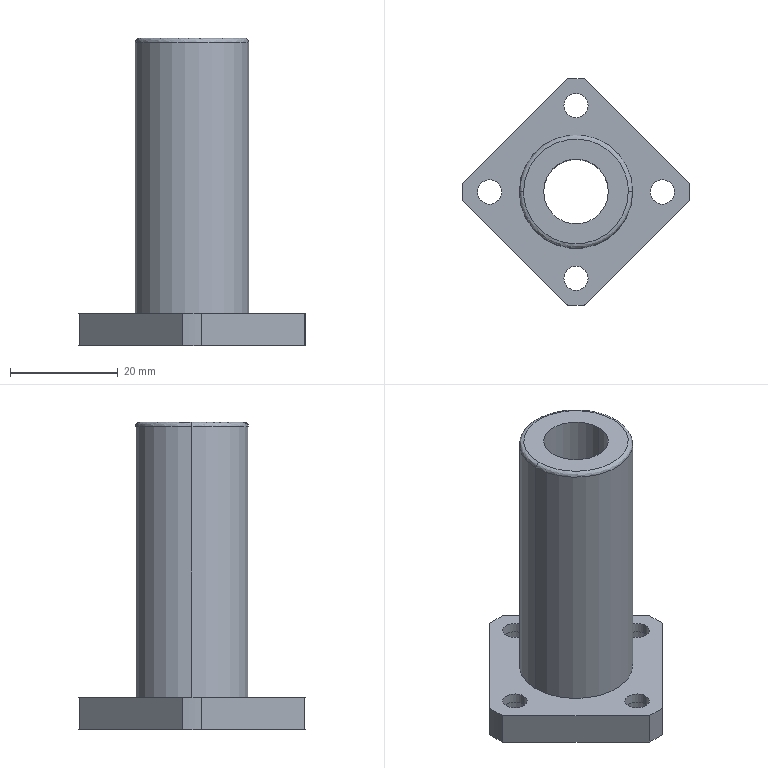Part | SolidWorks | features BaseBody 1 | 1 solid | 38 faces | box 42 x 42 x 57 mm | volume 16443 mm3 | cylinder 25 | plane 11 | spline 2 | commonest cylinder face diameters 4.5 x8 7.5 x8 42 x5 12 x2 21 x2
STEP:
#1=CARTESIAN_POINT('',(10.5,0.,56.2));
#2=VERTEX_POINT('',#1);
#3=CARTESIAN_POINT('',(-10.5,0.,56.2));
#4=VERTEX_POINT('',#3);
#5=CARTESIAN_POINT('',(0.,0.,56.2));
#6=DIRECTION('',(0.,0.,-1.));
#7=DIRECTION('',(1.,0.,0.));
#8=AXIS2_PLACEMENT_3D('',#5,#6,#7);
#9=CIRCLE('',#8,10.5);
#10=EDGE_CURVE('',#2,#4,#9,.T.);
#11=ORIENTED_EDGE('',*,*,#10,.F.);
#12=CARTESIAN_POINT('',(9.7,0.,57.));
#13=VERTEX_POINT('',#12);
#14=CARTESIAN_POINT('',(9.7,0.,56.2));
#15=DIRECTION('',(0.,-1.,0.));
#16=DIRECTION('',(1.,0.,0.));
#17=AXIS2_PLACEMENT_3D('',#14,#15,#16);
#18=CIRCLE('',#17,0.8);
#19=EDGE_CURVE('',#2,#13,#18,.T.);
#20=ORIENTED_EDGE('',*,*,#19,.T.);
#21=CARTESIAN_POINT('',(-9.7,0.,57.));
#22=VERTEX_POINT('',#21);
#23=CARTESIAN_POINT('',(9.7,0.,57.));
#24=CARTESIAN_POINT('',(9.7,-19.4,57.));
#25=CARTESIAN_POINT('',(-9.7,-19.4,57.));
#26=CARTESIAN_POINT('',(-9.7,0.,57.));
#27=(BOUNDED_CURVE()B_SPLINE_CURVE(3,(#23,#24,#25,#26),.UNSPECIFIED.,.F.,.F.)B_SPLINE_CURVE_WITH_KNOTS((4,4),(0.5,1.),.UNSPECIFIED.)CURVE()GEOMETRIC_REPRESENTATION_ITEM()RATIONAL_B_SPLINE_CURVE((1.,0.3333,0.3333,1.))REPRESENTATION_ITEM(''));
#28=EDGE_CURVE('',#13,#22,#27,.T.);
#29=ORIENTED_EDGE('',*,*,#28,.T.);
#30=CARTESIAN_POINT('',(-9.7,0.,56.2));
#31=DIRECTION('',(0.,1.,0.));
#32=DIRECTION('',(-1.,0.,0.));
#33=AXIS2_PLACEMENT_3D('',#30,#31,#32);
#34=CIRCLE('',#33,0.8);
#35=EDGE_CURVE('',#4,#22,#34,.T.);
#36=ORIENTED_EDGE('',*,*,#35,.F.);
#37=EDGE_LOOP('',(#11,#20,#29,#36));
#38=FACE_OUTER_BOUND('',#37,.T.);
#39=CARTESIAN_POINT('',(10.5,0.,56.2));
#40=CARTESIAN_POINT('',(10.5,-21.,56.2));
#41=CARTESIAN_POINT('',(-10.5,-21.,56.2));
#42=CARTESIAN_POINT('',(-10.5,0.,56.2));
#43=CARTESIAN_POINT('',(10.5,0.,56.669));
#44=CARTESIAN_POINT('',(10.5,-21.,56.669));
#45=CARTESIAN_POINT('',(-10.5,-21.,56.669));
#46=CARTESIAN_POINT('',(-10.5,0.,56.669));
#47=CARTESIAN_POINT('',(10.169,0.,57.));
#48=CARTESIAN_POINT('',(10.169,-20.337,57.));
#49=CARTESIAN_POINT('',(-10.169,-20.337,57.));
#50=CARTESIAN_POINT('',(-10.169,0.,57.));
#51=CARTESIAN_POINT('',(9.7,0.,57.));
#52=CARTESIAN_POINT('',(9.7,-19.4,57.));
#53=CARTESIAN_POINT('',(-9.7,-19.4,57.));
#54=CARTESIAN_POINT('',(-9.7,0.,57.));
#55=(BOUNDED_SURFACE()B_SPLINE_SURFACE(3,3,((#39,#40,#41,#42),(#43,#44,#45,#46),(#47,#48,#49,#50),(#51,#52,#53,#54)),.UNSPECIFIED.,.F.,.F.,.F.)B_SPLINE_SURFACE_WITH_KNOTS((4,4),(4,4),(0.,1.),(0.,1.),.UNSPECIFIED.)GEOMETRIC_REPRESENTATION_ITEM()RATIONAL_B_SPLINE_SURFACE(((1.,0.3333,0.3333,1.),(0.8047,0.2682,0.2682,0.8047),(0.8047,0.2682,0.2682,0.8047),(1.,0.3333,0.3333,1.)))REPRESENTATION_ITEM('')SURFACE());
#56=ADVANCED_FACE('',(#38),#55,.T.);
#57=CARTESIAN_POINT('',(10.5,0.,6.));
#58=VERTEX_POINT('',#57);
#59=CARTESIAN_POINT('',(-10.5,0.,6.));
#60=VERTEX_POINT('',#59);
#61=CARTESIAN_POINT('',(0.,0.,6.));
#62=DIRECTION('',(0.,0.,1.));
#63=DIRECTION('',(1.,0.,0.));
#64=AXIS2_PLACEMENT_3D('',#61,#62,#63);
#65=CIRCLE('',#64,10.5);
#66=EDGE_CURVE('',#58,#60,#65,.T.);
#67=ORIENTED_EDGE('',*,*,#66,.T.);
#68=CARTESIAN_POINT('',(-10.5,0.,0.));
#69=DIRECTION('',(0.,0.,1.));
#70=VECTOR('',#69,1000.);
#71=LINE('',#68,#70);
#72=EDGE_CURVE('',#60,#4,#71,.T.);
#73=ORIENTED_EDGE('',*,*,#72,.T.);
#74=CARTESIAN_POINT('',(0.,0.,56.2));
#75=DIRECTION('',(0.,0.,-1.));
#76=DIRECTION('',(1.,0.,0.));
#77=AXIS2_PLACEMENT_3D('',#74,#75,#76);
#78=CIRCLE('',#77,10.5);
#79=EDGE_CURVE('',#4,#2,#78,.T.);
#80=ORIENTED_EDGE('',*,*,#79,.T.);
#81=CARTESIAN_POINT('',(10.5,0.,0.));
#82=DIRECTION('',(0.,0.,1.));
#83=VECTOR('',#82,1000.);
#84=LINE('',#81,#83);
#85=EDGE_CURVE('',#58,#2,#84,.T.);
#86=ORIENTED_EDGE('',*,*,#85,.F.);
#87=EDGE_LOOP('',(#67,#73,#80,#86));
#88=FACE_OUTER_BOUND('',#87,.T.);
#89=CARTESIAN_POINT('',(0.,0.,0.));
#90=DIRECTION('',(0.,0.,1.));
#91=DIRECTION('',(1.,0.,0.));
#92=AXIS2_PLACEMENT_3D('',#89,#90,#91);
#93=CYLINDRICAL_SURFACE('',#92,10.5);
#94=ADVANCED_FACE('',(#88),#93,.T.);
#95=CARTESIAN_POINT('',(18.25,0.,6.));
#96=VERTEX_POINT('',#95);
#97=CARTESIAN_POINT('',(13.75,0.,6.));
#98=VERTEX_POINT('',#97);
#99=CARTESIAN_POINT('',(16.,0.,6.));
#100=DIRECTION('',(0.,0.,-1.));
#101=DIRECTION('',(-1.,0.,0.));
#102=AXIS2_PLACEMENT_3D('',#99,#100,#101);
#103=CIRCLE('',#102,2.25);
#104=EDGE_CURVE('',#96,#98,#103,.T.);
#105=ORIENTED_EDGE('',*,*,#104,.F.);
#106=CARTESIAN_POINT('',(18.25,0.,4.1));
#107=VERTEX_POINT('',#106);
#108=CARTESIAN_POINT('',(18.25,0.,6.));
#109=DIRECTION('',(0.,0.,-1.));
#110=VECTOR('',#109,1000.);
#111=LINE('',#108,#110);
#112=EDGE_CURVE('',#96,#107,#111,.T.);
#113=ORIENTED_EDGE('',*,*,#112,.T.);
#114=CARTESIAN_POINT('',(13.75,0.,4.1));
#115=VERTEX_POINT('',#114);
#116=CARTESIAN_POINT('',(16.,0.,4.1));
#117=DIRECTION('',(0.,0.,1.));
#118=DIRECTION('',(-1.,0.,0.));
#119=AXIS2_PLACEMENT_3D('',#116,#117,#118);
#120=CIRCLE('',#119,2.25);
#121=EDGE_CURVE('',#115,#107,#120,.T.);
#122=ORIENTED_EDGE('',*,*,#121,.F.);
#123=CARTESIAN_POINT('',(13.75,0.,6.));
#124=DIRECTION('',(0.,0.,-1.));
#125=VECTOR('',#124,1000.);
#126=LINE('',#123,#125);
#127=EDGE_CURVE('',#98,#115,#126,.T.);
#128=ORIENTED_EDGE('',*,*,#127,.F.);
#129=EDGE_LOOP('',(#105,#113,#122,#128));
#130=FACE_OUTER_BOUND('',#129,.T.);
#131=CARTESIAN_POINT('',(16.,0.,6.));
#132=DIRECTION('',(0.,0.,-1.));
#133=DIRECTION('',(-1.,0.,0.));
#134=AXIS2_PLACEMENT_3D('',#131,#132,#133);
#135=CYLINDRICAL_SURFACE('',#134,2.25);
#136=ADVANCED_FACE('',(#130),#135,.F.);
#137=CARTESIAN_POINT('',(2.25,-16.,6.));
#138=VERTEX_POINT('',#137);
#139=CARTESIAN_POINT('',(-2.25,-16.,6.));
#140=VERTEX_POINT('',#139);
#141=CARTESIAN_POINT('',(0.,-16.,6.));
#142=DIRECTION('',(0.,0.,-1.));
#143=DIRECTION('',(-1.,0.,0.));
#144=AXIS2_PLACEMENT_3D('',#141,#142,#143);
#145=CIRCLE('',#144,2.25);
#146=EDGE_CURVE('',#138,#140,#145,.T.);
#147=ORIENTED_EDGE('',*,*,#146,.F.);
#148=CARTESIAN_POINT('',(2.25,-16.,4.1));
#149=VERTEX_POINT('',#148);
#150=CARTESIAN_POINT('',(2.25,-16.,6.));
#151=DIRECTION('',(0.,0.,-1.));
#152=VECTOR('',#151,1000.);
#153=LINE('',#150,#152);
#154=EDGE_CURVE('',#138,#149,#153,.T.);
#155=ORIENTED_EDGE('',*,*,#154,.T.);
#156=CARTESIAN_POINT('',(-2.25,-16.,4.1));
#157=VERTEX_POINT('',#156);
#158=CARTESIAN_POINT('',(0.,-16.,4.1));
#159=DIRECTION('',(0.,0.,1.));
#160=DIRECTION('',(-1.,0.,0.));
#161=AXIS2_PLACEMENT_3D('',#158,#159,#160);
#162=CIRCLE('',#161,2.25);
#163=EDGE_CURVE('',#157,#149,#162,.T.);
#164=ORIENTED_EDGE('',*,*,#163,.F.);
#165=CARTESIAN_POINT('',(-2.25,-16.,6.));
#166=DIRECTION('',(0.,0.,-1.));
#167=VECTOR('',#166,1000.);
#168=LINE('',#165,#167);
#169=EDGE_CURVE('',#140,#157,#168,.T.);
#170=ORIENTED_EDGE('',*,*,#169,.F.);
#171=EDGE_LOOP('',(#147,#155,#164,#170));
#172=FACE_OUTER_BOUND('',#171,.T.);
#173=CARTESIAN_POINT('',(0.,-16.,6.));
#174=DIRECTION('',(0.,0.,-1.));
#175=DIRECTION('',(-1.,0.,0.));
#176=AXIS2_PLACEMENT_3D('',#173,#174,#175);
#177=CYLINDRICAL_SURFACE('',#176,2.25);
#178=ADVANCED_FACE('',(#172),#177,.F.);
#179=CARTESIAN_POINT('',(20.931,-1.696,0.));
#180=VERTEX_POINT('',#179);
#181=CARTESIAN_POINT('',(21.,0.,0.));
#182=VERTEX_POINT('',#181);
#183=CARTESIAN_POINT('',(0.,0.,0.));
#184=DIRECTION('',(0.,0.,1.));
#185=DIRECTION('',(1.,0.,0.));
#186=AXIS2_PLACEMENT_3D('',#183,#184,#185);
#187=CIRCLE('',#186,21.);
#188=EDGE_CURVE('',#180,#182,#187,.T.);
#189=ORIENTED_EDGE('',*,*,#188,.T.);
#190=CARTESIAN_POINT('',(21.,0.,6.));
#191=VERTEX_POINT('',#190);
#192=CARTESIAN_POINT('',(21.,0.,6.));
#193=DIRECTION('',(0.,0.,1.));
#194=VECTOR('',#193,1000.);
#195=LINE('',#192,#194);
#196=EDGE_CURVE('',#182,#191,#195,.T.);
#197=ORIENTED_EDGE('',*,*,#196,.T.);
#198=CARTESIAN_POINT('',(20.931,-1.696,6.));
#199=VERTEX_POINT('',#198);
#200=CARTESIAN_POINT('',(0.,0.,6.));
#201=DIRECTION('',(0.,0.,1.));
#202=DIRECTION('',(1.,0.,0.));
#203=AXIS2_PLACEMENT_3D('',#200,#201,#202);
#204=CIRCLE('',#203,21.);
#205=EDGE_CURVE('',#199,#191,#204,.T.);
#206=ORIENTED_EDGE('',*,*,#205,.F.);
#207=CARTESIAN_POINT('',(20.931,-1.696,6.));
#208=DIRECTION('',(0.,0.,-1.));
#209=VECTOR('',#208,1000.);
#210=LINE('',#207,#209);
#211=EDGE_CURVE('',#199,#180,#210,.T.);
#212=ORIENTED_EDGE('',*,*,#211,.T.);
#213=EDGE_LOOP('',(#189,#197,#206,#212));
#214=FACE_OUTER_BOUND('',#213,.T.);
#215=CARTESIAN_POINT('',(0.,0.,6.));
#216=DIRECTION('',(0.,0.,1.));
#217=DIRECTION('',(1.,0.,0.));
#218=AXIS2_PLACEMENT_3D('',#215,#216,#217);
#219=CYLINDRICAL_SURFACE('',#218,21.);
#220=ADVANCED_FACE('',(#214),#219,.T.);
#221=CARTESIAN_POINT('',(-2.25,16.,4.1));
#222=VERTEX_POINT('',#221);
#223=CARTESIAN_POINT('',(2.25,16.,4.1));
#224=VERTEX_POINT('',#223);
#225=CARTESIAN_POINT('',(0.,16.,4.1));
#226=DIRECTION('',(0.,0.,1.));
#227=DIRECTION('',(1.,0.,0.));
#228=AXIS2_PLACEMENT_3D('',#225,#226,#227);
#229=CIRCLE('',#228,2.25);
#230=EDGE_CURVE('',#222,#224,#229,.T.);
#231=ORIENTED_EDGE('',*,*,#230,.F.);
#232=CARTESIAN_POINT('',(-2.25,16.,6.));
#233=VERTEX_POINT('',#232);
#234=CARTESIAN_POINT('',(-2.25,16.,0.));
#235=DIRECTION('',(0.,0.,1.));
#236=VECTOR('',#235,1000.);
#237=LINE('',#234,#236);
#238=EDGE_CURVE('',#222,#233,#237,.T.);
#239=ORIENTED_EDGE('',*,*,#238,.T.);
#240=CARTESIAN_POINT('',(2.25,16.,6.));
#241=VERTEX_POINT('',#240);
#242=CARTESIAN_POINT('',(0.,16.,6.));
#243=DIRECTION('',(0.,0.,-1.));
#244=DIRECTION('',(1.,0.,0.));
#245=AXIS2_PLACEMENT_3D('',#242,#243,#244);
#246=CIRCLE('',#245,2.25);
#247=EDGE_CURVE('',#241,#233,#246,.T.);
#248=ORIENTED_EDGE('',*,*,#247,.F.);
#249=CARTESIAN_POINT('',(2.25,16.,0.));
#250=DIRECTION('',(0.,0.,1.));
#251=VECTOR('',#250,1000.);
#252=LINE('',#249,#251);
#253=EDGE_CURVE('',#224,#241,#252,.T.);
#254=ORIENTED_EDGE('',*,*,#253,.F.);
#255=EDGE_LOOP('',(#231,#239,#248,#254));
#256=FACE_OUTER_BOUND('',#255,.T.);
#257=CARTESIAN_POINT('',(0.,16.,0.));
#258=DIRECTION('',(0.,0.,1.));
#259=DIRECTION('',(1.,0.,0.));
#260=AXIS2_PLACEMENT_3D('',#257,#258,#259);
#261=CYLINDRICAL_SURFACE('',#260,2.25);
#262=ADVANCED_FACE('',(#256),#261,.F.);
#263=CARTESIAN_POINT('',(-18.25,0.,4.1));
#264=VERTEX_POINT('',#263);
#265=CARTESIAN_POINT('',(-13.75,0.,4.1));
#266=VERTEX_POINT('',#265);
#267=CARTESIAN_POINT('',(-16.,0.,4.1));
#268=DIRECTION('',(0.,0.,1.));
#269=DIRECTION('',(1.,0.,0.));
#270=AXIS2_PLACEMENT_3D('',#267,#268,#269);
#271=CIRCLE('',#270,2.25);
#272=EDGE_CURVE('',#264,#266,#271,.T.);
#273=ORIENTED_EDGE('',*,*,#272,.F.);
#274=CARTESIAN_POINT('',(-18.25,0.,6.));
#275=VERTEX_POINT('',#274);
#276=CARTESIAN_POINT('',(-18.25,0.,0.));
#277=DIRECTION('',(0.,0.,1.));
#278=VECTOR('',#277,1000.);
#279=LINE('',#276,#278);
#280=EDGE_CURVE('',#264,#275,#279,.T.);
#281=ORIENTED_EDGE('',*,*,#280,.T.);
#282=CARTESIAN_POINT('',(-13.75,0.,6.));
#283=VERTEX_POINT('',#282);
#284=CARTESIAN_POINT('',(-16.,0.,6.));
#285=DIRECTION('',(0.,0.,-1.));
#286=DIRECTION('',(1.,0.,0.));
#287=AXIS2_PLACEMENT_3D('',#284,#285,#286);
#288=CIRCLE('',#287,2.25);
#289=EDGE_CURVE('',#283,#275,#288,.T.);
#290=ORIENTED_EDGE('',*,*,#289,.F.);
#291=CARTESIAN_POINT('',(-13.75,0.,0.));
#292=DIRECTION('',(0.,0.,1.));
#293=VECTOR('',#292,1000.);
#294=LINE('',#291,#293);
#295=EDGE_CURVE('',#266,#283,#294,.T.);
#296=ORIENTED_EDGE('',*,*,#295,.F.);
#297=EDGE_LOOP('',(#273,#281,#290,#296));
#298=FACE_OUTER_BOUND('',#297,.T.);
#299=CARTESIAN_POINT('',(-16.,0.,0.));
#300=DIRECTION('',(0.,0.,1.));
#301=DIRECTION('',(1.,0.,0.));
#302=AXIS2_PLACEMENT_3D('',#299,#300,#301);
#303=CYLINDRICAL_SURFACE('',#302,2.25);
#304=ADVANCED_FACE('',(#298),#303,.F.);
#305=CARTESIAN_POINT('',(-6.,0.,0.));
#306=VERTEX_POINT('',#305);
#307=CARTESIAN_POINT('',(6.,0.,0.));
#308=VERTEX_POINT('',#307);
#309=CARTESIAN_POINT('',(0.,0.,0.));
#310=DIRECTION('',(0.,0.,1.));
#311=DIRECTION('',(1.,0.,0.));
#312=AXIS2_PLACEMENT_3D('',#309,#310,#311);
#313=CIRCLE('',#312,6.);
#314=EDGE_CURVE('',#306,#308,#313,.T.);
#315=ORIENTED_EDGE('',*,*,#314,.F.);
#316=CARTESIAN_POINT('',(-6.,0.,57.));
#317=VERTEX_POINT('',#316);
#318=CARTESIAN_POINT('',(-6.,0.,0.));
#319=DIRECTION('',(0.,0.,1.));
#320=VECTOR('',#319,1000.);
#321=LINE('',#318,#320);
#322=EDGE_CURVE('',#306,#317,#321,.T.);
#323=ORIENTED_EDGE('',*,*,#322,.T.);
#324=CARTESIAN_POINT('',(6.,0.,57.));
#325=VERTEX_POINT('',#324);
#326=CARTESIAN_POINT('',(0.,0.,57.));
#327=DIRECTION('',(0.,0.,-1.));
#328=DIRECTION('',(1.,0.,0.));
#329=AXIS2_PLACEMENT_3D('',#326,#327,#328);
#330=CIRCLE('',#329,6.);
#331=EDGE_CURVE('',#325,#317,#330,.T.);
#332=ORIENTED_EDGE('',*,*,#331,.F.);
#333=CARTESIAN_POINT('',(6.,0.,0.));
#334=DIRECTION('',(0.,0.,1.));
#335=VECTOR('',#334,1000.);
#336=LINE('',#333,#335);
#337=EDGE_CURVE('',#308,#325,#336,.T.);
#338=ORIENTED_EDGE('',*,*,#337,.F.);
#339=EDGE_LOOP('',(#315,#323,#332,#338));
#340=FACE_OUTER_BOUND('',#339,.T.);
#341=CARTESIAN_POINT('',(0.,0.,0.));
#342=DIRECTION('',(0.,0.,1.));
#343=DIRECTION('',(1.,0.,0.));
#344=AXIS2_PLACEMENT_3D('',#341,#342,#343);
#345=CYLINDRICAL_SURFACE('',#344,6.);
#346=ADVANCED_FACE('',(#340),#345,.F.);
#347=CARTESIAN_POINT('',(19.75,0.,4.1));
#348=VERTEX_POINT('',#347);
#349=CARTESIAN_POINT('',(12.25,0.,4.1));
#350=VERTEX_POINT('',#349);
#351=CARTESIAN_POINT('',(16.,0.,4.1));
#352=DIRECTION('',(0.,0.,-1.));
#353=DIRECTION('',(-1.,0.,0.));
#354=AXIS2_PLACEMENT_3D('',#351,#352,#353);
#355=CIRCLE('',#354,3.75);
#356=EDGE_CURVE('',#348,#350,#355,.T.);
#357=ORIENTED_EDGE('',*,*,#356,.F.);
#358=CARTESIAN_POINT('',(19.75,0.,0.));
#359=VERTEX_POINT('',#358);
#360=CARTESIAN_POINT('',(19.75,0.,6.));
#361=DIRECTION('',(0.,0.,-1.));
#362=VECTOR('',#361,1000.);
#363=LINE('',#360,#362);
#364=EDGE_CURVE('',#348,#359,#363,.T.);
#365=ORIENTED_EDGE('',*,*,#364,.T.);
#366=CARTESIAN_POINT('',(12.25,0.,0.));
#367=VERTEX_POINT('',#366);
#368=CARTESIAN_POINT('',(16.,0.,0.));
#369=DIRECTION('',(0.,0.,1.));
#370=DIRECTION('',(-1.,0.,0.));
#371=AXIS2_PLACEMENT_3D('',#368,#369,#370);
#372=CIRCLE('',#371,3.75);
#373=EDGE_CURVE('',#367,#359,#372,.T.);
#374=ORIENTED_EDGE('',*,*,#373,.F.);
#375=CARTESIAN_POINT('',(12.25,0.,6.));
#376=DIRECTION('',(0.,0.,-1.));
#377=VECTOR('',#376,1000.);
#378=LINE('',#375,#377);
#379=EDGE_CURVE('',#350,#367,#378,.T.);
#380=ORIENTED_EDGE('',*,*,#379,.F.);
#381=EDGE_LOOP('',(#357,#365,#374,#380));
#382=FACE_OUTER_BOUND('',#381,.T.);
#383=CARTESIAN_POINT('',(16.,0.,6.));
#384=DIRECTION('',(0.,0.,-1.));
#385=DIRECTION('',(-1.,0.,0.));
#386=AXIS2_PLACEMENT_3D('',#383,#384,#385);
#387=CYLINDRICAL_SURFACE('',#386,3.75);
#388=ADVANCED_FACE('',(#382),#387,.F.);
#389=CARTESIAN_POINT('',(3.75,-16.,4.1));
#390=VERTEX_POINT('',#389);
#391=CARTESIAN_POINT('',(-3.75,-16.,4.1));
#392=VERTEX_POINT('',#391);
#393=CARTESIAN_POINT('',(0.,-16.,4.1));
#394=DIRECTION('',(0.,0.,-1.));
#395=DIRECTION('',(-1.,0.,0.));
#396=AXIS2_PLACEMENT_3D('',#393,#394,#395);
#397=CIRCLE('',#396,3.75);
#398=EDGE_CURVE('',#390,#392,#397,.T.);
#399=ORIENTED_EDGE('',*,*,#398,.F.);
#400=CARTESIAN_POINT('',(3.75,-16.,0.));
#401=VERTEX_POINT('',#400);
#402=CARTESIAN_POINT('',(3.75,-16.,6.));
#403=DIRECTION('',(0.,0.,-1.));
#404=VECTOR('',#403,1000.);
#405=LINE('',#402,#404);
#406=EDGE_CURVE('',#390,#401,#405,.T.);
#407=ORIENTED_EDGE('',*,*,#406,.T.);
#408=CARTESIAN_POINT('',(-3.75,-16.,0.));
#409=VERTEX_POINT('',#408);
#410=CARTESIAN_POINT('',(0.,-16.,0.));
#411=DIRECTION('',(0.,0.,1.));
#412=DIRECTION('',(-1.,0.,0.));
#413=AXIS2_PLACEMENT_3D('',#410,#411,#412);
#414=CIRCLE('',#413,3.75);
#415=EDGE_CURVE('',#409,#401,#414,.T.);
#416=ORIENTED_EDGE('',*,*,#415,.F.);
#417=CARTESIAN_POINT('',(-3.75,-16.,6.));
#418=DIRECTION('',(0.,0.,-1.));
#419=VECTOR('',#418,1000.);
#420=LINE('',#417,#419);
#421=EDGE_CURVE('',#392,#409,#420,.T.);
#422=ORIENTED_EDGE('',*,*,#421,.F.);
#423=EDGE_LOOP('',(#399,#407,#416,#422));
#424=FACE_OUTER_BOUND('',#423,.T.);
#425=CARTESIAN_POINT('',(0.,-16.,6.));
#426=DIRECTION('',(0.,0.,-1.));
#427=DIRECTION('',(-1.,0.,0.));
#428=AXIS2_PLACEMENT_3D('',#425,#426,#427);
#429=CYLINDRICAL_SURFACE('',#428,3.75);
#430=ADVANCED_FACE('',(#424),#429,.F.);
#431=CARTESIAN_POINT('',(-3.75,16.,0.));
#432=VERTEX_POINT('',#431);
#433=CARTESIAN_POINT('',(3.75,16.,0.));
#434=VERTEX_POINT('',#433);
#435=CARTESIAN_POINT('',(0.,16.,0.));
#436=DIRECTION('',(0.,0.,1.));
#437=DIRECTION('',(1.,0.,0.));
#438=AXIS2_PLACEMENT_3D('',#435,#436,#437);
#439=CIRCLE('',#438,3.75);
#440=EDGE_CURVE('',#432,#434,#439,.T.);
#441=ORIENTED_EDGE('',*,*,#440,.F.);
#442=CARTESIAN_POINT('',(-3.75,16.,4.1));
#443=VERTEX_POINT('',#442);
#444=CARTESIAN_POINT('',(-3.75,16.,0.));
#445=DIRECTION('',(0.,0.,1.));
#446=VECTOR('',#445,1000.);
#447=LINE('',#444,#446);
#448=EDGE_CURVE('',#432,#443,#447,.T.);
#449=ORIENTED_EDGE('',*,*,#448,.T.);
#450=CARTESIAN_POINT('',(3.75,16.,4.1));
#451=VERTEX_POINT('',#450);
#452=CARTESIAN_POINT('',(0.,16.,4.1));
#453=DIRECTION('',(0.,0.,-1.));
#454=DIRECTION('',(1.,0.,0.));
#455=AXIS2_PLACEMENT_3D('',#452,#453,#454);
#456=CIRCLE('',#455,3.75);
#457=EDGE_CURVE('',#451,#443,#456,.T.);
#458=ORIENTED_EDGE('',*,*,#457,.F.);
#459=CARTESIAN_POINT('',(3.75,16.,0.));
#460=DIRECTION('',(0.,0.,1.));
#461=VECTOR('',#460,1000.);
#462=LINE('',#459,#461);
#463=EDGE_CURVE('',#434,#451,#462,.T.);
#464=ORIENTED_EDGE('',*,*,#463,.F.);
#465=EDGE_LOOP('',(#441,#449,#458,#464));
#466=FACE_OUTER_BOUND('',#465,.T.);
#467=CARTESIAN_POINT('',(0.,16.,0.));
#468=DIRECTION('',(0.,0.,1.));
#469=DIRECTION('',(1.,0.,0.));
#470=AXIS2_PLACEMENT_3D('',#467,#468,#469);
#471=CYLINDRICAL_SURFACE('',#470,3.75);
#472=ADVANCED_FACE('',(#466),#471,.F.);
#473=CARTESIAN_POINT('',(-19.75,0.,0.));
#474=VERTEX_POINT('',#473);
#475=CARTESIAN_POINT('',(-12.25,0.,0.));
#476=VERTEX_POINT('',#475);
#477=CARTESIAN_POINT('',(-16.,0.,0.));
#478=DIRECTION('',(0.,0.,1.));
#479=DIRECTION('',(1.,0.,0.));
#480=AXIS2_PLACEMENT_3D('',#477,#478,#479);
#481=CIRCLE('',#480,3.75);
#482=EDGE_CURVE('',#474,#476,#481,.T.);
#483=ORIENTED_EDGE('',*,*,#482,.F.);
#484=CARTESIAN_POINT('',(-19.75,0.,4.1));
#485=VERTEX_POINT('',#484);
#486=CARTESIAN_POINT('',(-19.75,0.,0.));
#487=DIRECTION('',(0.,0.,1.));
#488=VECTOR('',#487,1000.);
#489=LINE('',#486,#488);
#490=EDGE_CURVE('',#474,#485,#489,.T.);
#491=ORIENTED_EDGE('',*,*,#490,.T.);
#492=CARTESIAN_POINT('',(-12.25,0.,4.1));
#493=VERTEX_POINT('',#492);
#494=CARTESIAN_POINT('',(-16.,0.,4.1));
#495=DIRECTION('',(0.,0.,-1.));
#496=DIRECTION('',(1.,0.,0.));
#497=AXIS2_PLACEMENT_3D('',#494,#495,#496);
#498=CIRCLE('',#497,3.75);
#499=EDGE_CURVE('',#493,#485,#498,.T.);
#500=ORIENTED_EDGE('',*,*,#499,.F.);
#501=CARTESIAN_POINT('',(-12.25,0.,0.));
#502=DIRECTION('',(0.,0.,1.));
#503=VECTOR('',#502,1000.);
#504=LINE('',#501,#503);
#505=EDGE_CURVE('',#476,#493,#504,.T.);
#506=ORIENTED_EDGE('',*,*,#505,.F.);
#507=EDGE_LOOP('',(#483,#491,#500,#506));
#508=FACE_OUTER_BOUND('',#507,.T.);
#509=CARTESIAN_POINT('',(-16.,0.,0.));
#510=DIRECTION('',(0.,0.,1.));
#511=DIRECTION('',(1.,0.,0.));
#512=AXIS2_PLACEMENT_3D('',#509,#510,#511);
#513=CYLINDRICAL_SURFACE('',#512,3.75);
#514=ADVANCED_FACE('',(#508),#513,.F.);
#515=ORIENTED_EDGE('',*,*,#72,.F.);
#516=CARTESIAN_POINT('',(0.,0.,6.));
#517=DIRECTION('',(0.,0.,1.));
#518=DIRECTION('',(1.,0.,0.));
#519=AXIS2_PLACEMENT_3D('',#516,#517,#518);
#520=CIRCLE('',#519,10.5);
#521=EDGE_CURVE('',#60,#58,#520,.T.);
#522=ORIENTED_EDGE('',*,*,#521,.T.);
#523=ORIENTED_EDGE('',*,*,#85,.T.);
#524=ORIENTED_EDGE('',*,*,#10,.T.);
#525=EDGE_LOOP('',(#515,#522,#523,#524));
#526=FACE_OUTER_BOUND('',#525,.T.);
#527=CARTESIAN_POINT('',(0.,0.,0.));
#528=DIRECTION('',(0.,0.,1.));
#529=DIRECTION('',(1.,0.,0.));
#530=AXIS2_PLACEMENT_3D('',#527,#528,#529);
#531=CYLINDRICAL_SURFACE('',#530,10.5);
#532=ADVANCED_FACE('',(#526),#531,.T.);
#533=CARTESIAN_POINT('',(16.,0.,6.));
#534=DIRECTION('',(0.,0.,-1.));
#535=DIRECTION('',(-1.,0.,0.));
#536=AXIS2_PLACEMENT_3D('',#533,#534,#535);
#537=CIRCLE('',#536,2.25);
#538=EDGE_CURVE('',#98,#96,#537,.T.);
#539=ORIENTED_EDGE('',*,*,#538,.T.);
#540=ORIENTED_EDGE('',*,*,#104,.T.);
#541=EDGE_LOOP('',(#539,#540));
#542=FACE_BOUND('',#541,.T.);
#543=CARTESIAN_POINT('',(0.,-16.,6.));
#544=DIRECTION('',(0.,0.,-1.));
#545=DIRECTION('',(-1.,0.,0.));
#546=AXIS2_PLACEMENT_3D('',#543,#544,#545);
#547=CIRCLE('',#546,2.25);
#548=EDGE_CURVE('',#140,#138,#547,.T.);
#549=ORIENTED_EDGE('',*,*,#548,.T.);
#550=ORIENTED_EDGE('',*,*,#146,.T.);
#551=EDGE_LOOP('',(#549,#550));
#552=FACE_BOUND('',#551,.T.);
#553=CARTESIAN_POINT('',(20.931,1.696,6.));
#554=VERTEX_POINT('',#553);
#555=CARTESIAN_POINT('',(1.696,20.931,6.));
#556=VERTEX_POINT('',#555);
#557=CARTESIAN_POINT('',(20.931,1.696,6.));
#558=DIRECTION('',(-0.7071,0.7071,0.));
#559=VECTOR('',#558,1000.);
#560=LINE('',#557,#559);
#561=EDGE_CURVE('',#554,#556,#560,.T.);
#562=ORIENTED_EDGE('',*,*,#561,.T.);
#563=CARTESIAN_POINT('',(-1.696,20.931,6.));
#564=VERTEX_POINT('',#563);
#565=CARTESIAN_POINT('',(0.,0.,6.));
#566=DIRECTION('',(0.,0.,1.));
#567=DIRECTION('',(1.,0.,0.));
#568=AXIS2_PLACEMENT_3D('',#565,#566,#567);
#569=CIRCLE('',#568,21.);
#570=EDGE_CURVE('',#556,#564,#569,.T.);
#571=ORIENTED_EDGE('',*,*,#570,.T.);
#572=CARTESIAN_POINT('',(-20.931,1.696,6.));
#573=VERTEX_POINT('',#572);
#574=CARTESIAN_POINT('',(-1.696,20.931,6.));
#575=DIRECTION('',(-0.7071,-0.7071,0.));
#576=VECTOR('',#575,1000.);
#577=LINE('',#574,#576);
#578=EDGE_CURVE('',#564,#573,#577,.T.);
#579=ORIENTED_EDGE('',*,*,#578,.T.);
#580=CARTESIAN_POINT('',(-20.931,-1.696,6.));
#581=VERTEX_POINT('',#580);
#582=CARTESIAN_POINT('',(0.,0.,6.));
#583=DIRECTION('',(0.,0.,1.));
#584=DIRECTION('',(1.,0.,0.));
#585=AXIS2_PLACEMENT_3D('',#582,#583,#584);
#586=CIRCLE('',#585,21.);
#587=EDGE_CURVE('',#573,#581,#586,.T.);
#588=ORIENTED_EDGE('',*,*,#587,.T.);
#589=CARTESIAN_POINT('',(-1.696,-20.931,6.));
#590=VERTEX_POINT('',#589);
#591=CARTESIAN_POINT('',(-20.931,-1.696,6.));
#592=DIRECTION('',(0.7071,-0.7071,0.));
#593=VECTOR('',#592,1000.);
#594=LINE('',#591,#593);
#595=EDGE_CURVE('',#581,#590,#594,.T.);
#596=ORIENTED_EDGE('',*,*,#595,.T.);
#597=CARTESIAN_POINT('',(1.696,-20.931,6.));
#598=VERTEX_POINT('',#597);
#599=CARTESIAN_POINT('',(0.,0.,6.));
#600=DIRECTION('',(0.,0.,1.));
#601=DIRECTION('',(1.,0.,0.));
#602=AXIS2_PLACEMENT_3D('',#599,#600,#601);
#603=CIRCLE('',#602,21.);
#604=EDGE_CURVE('',#590,#598,#603,.T.);
#605=ORIENTED_EDGE('',*,*,#604,.T.);
#606=CARTESIAN_POINT('',(1.696,-20.931,6.));
#607=DIRECTION('',(0.7071,0.7071,0.));
#608=VECTOR('',#607,1000.);
#609=LINE('',#606,#608);
#610=EDGE_CURVE('',#598,#199,#609,.T.);
#611=ORIENTED_EDGE('',*,*,#610,.T.);
#612=ORIENTED_EDGE('',*,*,#205,.T.);
#613=CARTESIAN_POINT('',(0.,0.,6.));
#614=DIRECTION('',(0.,0.,1.));
#615=DIRECTION('',(1.,0.,0.));
#616=AXIS2_PLACEMENT_3D('',#613,#614,#615);
#617=CIRCLE('',#616,21.);
#618=EDGE_CURVE('',#191,#554,#617,.T.);
#619=ORIENTED_EDGE('',*,*,#618,.T.);
#620=EDGE_LOOP('',(#562,#571,#579,#588,#596,#605,#611,#612,#619));
#621=FACE_OUTER_BOUND('',#620,.T.);
#622=ORIENTED_EDGE('',*,*,#66,.F.);
#623=ORIENTED_EDGE('',*,*,#521,.F.);
#624=EDGE_LOOP('',(#622,#623));
#625=FACE_BOUND('',#624,.T.);
#626=ORIENTED_EDGE('',*,*,#247,.T.);
#627=CARTESIAN_POINT('',(0.,16.,6.));
#628=DIRECTION('',(0.,0.,-1.));
#629=DIRECTION('',(1.,0.,0.));
#630=AXIS2_PLACEMENT_3D('',#627,#628,#629);
#631=CIRCLE('',#630,2.25);
#632=EDGE_CURVE('',#233,#241,#631,.T.);
#633=ORIENTED_EDGE('',*,*,#632,.T.);
#634=EDGE_LOOP('',(#626,#633));
#635=FACE_BOUND('',#634,.T.);
#636=ORIENTED_EDGE('',*,*,#289,.T.);
#637=CARTESIAN_POINT('',(-16.,0.,6.));
#638=DIRECTION('',(0.,0.,-1.));
#639=DIRECTION('',(1.,0.,0.));
#640=AXIS2_PLACEMENT_3D('',#637,#638,#639);
#641=CIRCLE('',#640,2.25);
#642=EDGE_CURVE('',#275,#283,#641,.T.);
#643=ORIENTED_EDGE('',*,*,#642,.T.);
#644=EDGE_LOOP('',(#636,#643));
#645=FACE_BOUND('',#644,.T.);
#646=CARTESIAN_POINT('',(0.,0.,6.));
#647=DIRECTION('',(0.,0.,1.));
#648=DIRECTION('',(1.,0.,0.));
#649=AXIS2_PLACEMENT_3D('',#646,#647,#648);
#650=PLANE('',#649);
#651=ADVANCED_FACE('',(#542,#552,#621,#625,#635,#645),#650,.T.);
#652=ORIENTED_EDGE('',*,*,#19,.F.);
#653=ORIENTED_EDGE('',*,*,#79,.F.);
#654=ORIENTED_EDGE('',*,*,#35,.T.);
#655=CARTESIAN_POINT('',(-9.7,0.,57.));
#656=CARTESIAN_POINT('',(-9.7,19.4,57.));
#657=CARTESIAN_POINT('',(9.7,19.4,57.));
#658=CARTESIAN_POINT('',(9.7,0.,57.));
#659=(BOUNDED_CURVE()B_SPLINE_CURVE(3,(#655,#656,#657,#658),.UNSPECIFIED.,.F.,.F.)B_SPLINE_CURVE_WITH_KNOTS((4,4),(0.,0.5),.UNSPECIFIED.)CURVE()GEOMETRIC_REPRESENTATION_ITEM()RATIONAL_B_SPLINE_CURVE((1.,0.3333,0.3333,1.))REPRESENTATION_ITEM(''));
#660=EDGE_CURVE('',#22,#13,#659,.T.);
#661=ORIENTED_EDGE('',*,*,#660,.T.);
#662=EDGE_LOOP('',(#652,#653,#654,#661));
#663=FACE_OUTER_BOUND('',#662,.T.);
#664=CARTESIAN_POINT('',(-10.5,0.,56.2));
#665=CARTESIAN_POINT('',(-10.5,21.,56.2));
#666=CARTESIAN_POINT('',(10.5,21.,56.2));
#667=CARTESIAN_POINT('',(10.5,0.,56.2));
#668=CARTESIAN_POINT('',(-10.5,0.,56.669));
#669=CARTESIAN_POINT('',(-10.5,21.,56.669));
#670=CARTESIAN_POINT('',(10.5,21.,56.669));
#671=CARTESIAN_POINT('',(10.5,0.,56.669));
#672=CARTESIAN_POINT('',(-10.169,0.,57.));
#673=CARTESIAN_POINT('',(-10.169,20.337,57.));
#674=CARTESIAN_POINT('',(10.169,20.337,57.));
#675=CARTESIAN_POINT('',(10.169,0.,57.));
#676=CARTESIAN_POINT('',(-9.7,0.,57.));
#677=CARTESIAN_POINT('',(-9.7,19.4,57.));
#678=CARTESIAN_POINT('',(9.7,19.4,57.));
#679=CARTESIAN_POINT('',(9.7,0.,57.));
#680=(BOUNDED_SURFACE()B_SPLINE_SURFACE(3,3,((#664,#665,#666,#667),(#668,#669,#670,#671),(#672,#673,#674,#675),(#676,#677,#678,#679)),.UNSPECIFIED.,.F.,.F.,.F.)B_SPLINE_SURFACE_WITH_KNOTS((4,4),(4,4),(0.,1.),(0.,1.),.UNSPECIFIED.)GEOMETRIC_REPRESENTATION_ITEM()RATIONAL_B_SPLINE_SURFACE(((1.,0.3333,0.3333,1.),(0.8047,0.2682,0.2682,0.8047),(0.8047,0.2682,0.2682,0.8047),(1.,0.3333,0.3333,1.)))REPRESENTATION_ITEM('')SURFACE());
#681=ADVANCED_FACE('',(#663),#680,.T.);
#682=ORIENTED_EDGE('',*,*,#112,.F.);
#683=ORIENTED_EDGE('',*,*,#538,.F.);
#684=ORIENTED_EDGE('',*,*,#127,.T.);
#685=CARTESIAN_POINT('',(16.,0.,4.1));
#686=DIRECTION('',(0.,0.,1.));
#687=DIRECTION('',(-1.,0.,0.));
#688=AXIS2_PLACEMENT_3D('',#685,#686,#687);
#689=CIRCLE('',#688,2.25);
#690=EDGE_CURVE('',#107,#115,#689,.T.);
#691=ORIENTED_EDGE('',*,*,#690,.F.);
#692=EDGE_LOOP('',(#682,#683,#684,#691));
#693=FACE_OUTER_BOUND('',#692,.T.);
#694=CARTESIAN_POINT('',(16.,0.,6.));
#695=DIRECTION('',(0.,0.,-1.));
#696=DIRECTION('',(-1.,0.,0.));
#697=AXIS2_PLACEMENT_3D('',#694,#695,#696);
#698=CYLINDRICAL_SURFACE('',#697,2.25);
#699=ADVANCED_FACE('',(#693),#698,.F.);
#700=ORIENTED_EDGE('',*,*,#154,.F.);
#701=ORIENTED_EDGE('',*,*,#548,.F.);
#702=ORIENTED_EDGE('',*,*,#169,.T.);
#703=CARTESIAN_POINT('',(0.,-16.,4.1));
#704=DIRECTION('',(0.,0.,1.));
#705=DIRECTION('',(-1.,0.,0.));
#706=AXIS2_PLACEMENT_3D('',#703,#704,#705);
#707=CIRCLE('',#706,2.25);
#708=EDGE_CURVE('',#149,#157,#707,.T.);
#709=ORIENTED_EDGE('',*,*,#708,.F.);
#710=EDGE_LOOP('',(#700,#701,#702,#709));
#711=FACE_OUTER_BOUND('',#710,.T.);
#712=CARTESIAN_POINT('',(0.,-16.,6.));
#713=DIRECTION('',(0.,0.,-1.));
#714=DIRECTION('',(-1.,0.,0.));
#715=AXIS2_PLACEMENT_3D('',#712,#713,#714);
#716=CYLINDRICAL_SURFACE('',#715,2.25);
#717=ADVANCED_FACE('',(#711),#716,.F.);
#718=ORIENTED_EDGE('',*,*,#570,.F.);
#719=CARTESIAN_POINT('',(1.696,20.931,0.));
#720=VERTEX_POINT('',#719);
#721=CARTESIAN_POINT('',(1.696,20.931,6.));
#722=DIRECTION('',(0.,0.,-1.));
#723=VECTOR('',#722,1000.);
#724=LINE('',#721,#723);
#725=EDGE_CURVE('',#556,#720,#724,.T.);
#726=ORIENTED_EDGE('',*,*,#725,.T.);
#727=CARTESIAN_POINT('',(-1.696,20.931,0.));
#728=VERTEX_POINT('',#727);
#729=CARTESIAN_POINT('',(0.,0.,0.));
#730=DIRECTION('',(0.,0.,1.));
#731=DIRECTION('',(1.,0.,0.));
#732=AXIS2_PLACEMENT_3D('',#729,#730,#731);
#733=CIRCLE('',#732,21.);
#734=EDGE_CURVE('',#720,#728,#733,.T.);
#735=ORIENTED_EDGE('',*,*,#734,.T.);
#736=CARTESIAN_POINT('',(-1.696,20.931,6.));
#737=DIRECTION('',(0.,0.,1.));
#738=VECTOR('',#737,1000.);
#739=LINE('',#736,#738);
#740=EDGE_CURVE('',#728,#564,#739,.T.);
#741=ORIENTED_EDGE('',*,*,#740,.T.);
#742=EDGE_LOOP('',(#718,#726,#735,#741));
#743=FACE_OUTER_BOUND('',#742,.T.);
#744=CARTESIAN_POINT('',(0.,0.,6.));
#745=DIRECTION('',(0.,0.,1.));
#746=DIRECTION('',(1.,0.,0.));
#747=AXIS2_PLACEMENT_3D('',#744,#745,#746);
#748=CYLINDRICAL_SURFACE('',#747,21.);
#749=ADVANCED_FACE('',(#743),#748,.T.);
#750=ORIENTED_EDGE('',*,*,#725,.F.);
#751=ORIENTED_EDGE('',*,*,#561,.F.);
#752=CARTESIAN_POINT('',(20.931,1.696,0.));
#753=VERTEX_POINT('',#752);
#754=CARTESIAN_POINT('',(20.931,1.696,6.));
#755=DIRECTION('',(0.,0.,1.));
#756=VECTOR('',#755,1000.);
#757=LINE('',#754,#756);
#758=EDGE_CURVE('',#753,#554,#757,.T.);
#759=ORIENTED_EDGE('',*,*,#758,.F.);
#760=CARTESIAN_POINT('',(20.931,1.696,0.));
#761=DIRECTION('',(0.7071,-0.7071,0.));
#762=VECTOR('',#761,1000.);
#763=LINE('',#760,#762);
#764=EDGE_CURVE('',#720,#753,#763,.T.);
#765=ORIENTED_EDGE('',*,*,#764,.F.);
#766=EDGE_LOOP('',(#750,#751,#759,#765));
#767=FACE_OUTER_BOUND('',#766,.T.);
#768=CARTESIAN_POINT('',(20.931,1.696,6.));
#769=DIRECTION('',(-0.7071,-0.7071,0.));
#770=DIRECTION('',(0.7071,-0.7071,0.));
#771=AXIS2_PLACEMENT_3D('',#768,#769,#770);
#772=PLANE('',#771);
#773=ADVANCED_FACE('',(#767),#772,.F.);
#774=ORIENTED_EDGE('',*,*,#196,.F.);
#775=CARTESIAN_POINT('',(0.,0.,0.));
#776=DIRECTION('',(0.,0.,1.));
#777=DIRECTION('',(1.,0.,0.));
#778=AXIS2_PLACEMENT_3D('',#775,#776,#777);
#779=CIRCLE('',#778,21.);
#780=EDGE_CURVE('',#182,#753,#779,.T.);
#781=ORIENTED_EDGE('',*,*,#780,.T.);
#782=ORIENTED_EDGE('',*,*,#758,.T.);
#783=ORIENTED_EDGE('',*,*,#618,.F.);
#784=EDGE_LOOP('',(#774,#781,#782,#783));
#785=FACE_OUTER_BOUND('',#784,.T.);
#786=CARTESIAN_POINT('',(0.,0.,6.));
#787=DIRECTION('',(0.,0.,1.));
#788=DIRECTION('',(1.,0.,0.));
#789=AXIS2_PLACEMENT_3D('',#786,#787,#788);
#790=CYLINDRICAL_SURFACE('',#789,21.);
#791=ADVANCED_FACE('',(#785),#790,.T.);
#792=ORIENTED_EDGE('',*,*,#211,.F.);
#793=ORIENTED_EDGE('',*,*,#610,.F.);
#794=CARTESIAN_POINT('',(1.696,-20.931,0.));
#795=VERTEX_POINT('',#794);
#796=CARTESIAN_POINT('',(1.696,-20.931,6.));
#797=DIRECTION('',(0.,0.,1.));
#798=VECTOR('',#797,1000.);
#799=LINE('',#796,#798);
#800=EDGE_CURVE('',#795,#598,#799,.T.);
#801=ORIENTED_EDGE('',*,*,#800,.F.);
#802=CARTESIAN_POINT('',(1.696,-20.931,0.));
#803=DIRECTION('',(-0.7071,-0.7071,0.));
#804=VECTOR('',#803,1000.);
#805=LINE('',#802,#804);
#806=EDGE_CURVE('',#180,#795,#805,.T.);
#807=ORIENTED_EDGE('',*,*,#806,.F.);
#808=EDGE_LOOP('',(#792,#793,#801,#807));
#809=FACE_OUTER_BOUND('',#808,.T.);
#810=CARTESIAN_POINT('',(1.696,-20.931,6.));
#811=DIRECTION('',(-0.7071,0.7071,0.));
#812=DIRECTION('',(-0.7071,-0.7071,0.));
#813=AXIS2_PLACEMENT_3D('',#810,#811,#812);
#814=PLANE('',#813);
#815=ADVANCED_FACE('',(#809),#814,.F.);
#816=ORIENTED_EDGE('',*,*,#604,.F.);
#817=CARTESIAN_POINT('',(-1.696,-20.931,0.));
#818=VERTEX_POINT('',#817);
#819=CARTESIAN_POINT('',(-1.696,-20.931,6.));
#820=DIRECTION('',(0.,0.,-1.));
#821=VECTOR('',#820,1000.);
#822=LINE('',#819,#821);
#823=EDGE_CURVE('',#590,#818,#822,.T.);
#824=ORIENTED_EDGE('',*,*,#823,.T.);
#825=CARTESIAN_POINT('',(0.,0.,0.));
#826=DIRECTION('',(0.,0.,1.));
#827=DIRECTION('',(1.,0.,0.));
#828=AXIS2_PLACEMENT_3D('',#825,#826,#827);
#829=CIRCLE('',#828,21.);
#830=EDGE_CURVE('',#818,#795,#829,.T.);
#831=ORIENTED_EDGE('',*,*,#830,.T.);
#832=ORIENTED_EDGE('',*,*,#800,.T.);
#833=EDGE_LOOP('',(#816,#824,#831,#832));
#834=FACE_OUTER_BOUND('',#833,.T.);
#835=CARTESIAN_POINT('',(0.,0.,6.));
#836=DIRECTION('',(0.,0.,1.));
#837=DIRECTION('',(1.,0.,0.));
#838=AXIS2_PLACEMENT_3D('',#835,#836,#837);
#839=CYLINDRICAL_SURFACE('',#838,21.);
#840=ADVANCED_FACE('',(#834),#839,.T.);
#841=ORIENTED_EDGE('',*,*,#823,.F.);
#842=ORIENTED_EDGE('',*,*,#595,.F.);
#843=CARTESIAN_POINT('',(-20.931,-1.696,0.));
#844=VERTEX_POINT('',#843);
#845=CARTESIAN_POINT('',(-20.931,-1.696,6.));
#846=DIRECTION('',(0.,0.,1.));
#847=VECTOR('',#846,1000.);
#848=LINE('',#845,#847);
#849=EDGE_CURVE('',#844,#581,#848,.T.);
#850=ORIENTED_EDGE('',*,*,#849,.F.);
#851=CARTESIAN_POINT('',(-20.931,-1.696,0.));
#852=DIRECTION('',(-0.7071,0.7071,0.));
#853=VECTOR('',#852,1000.);
#854=LINE('',#851,#853);
#855=EDGE_CURVE('',#818,#844,#854,.T.);
#856=ORIENTED_EDGE('',*,*,#855,.F.);
#857=EDGE_LOOP('',(#841,#842,#850,#856));
#858=FACE_OUTER_BOUND('',#857,.T.);
#859=CARTESIAN_POINT('',(-20.931,-1.696,6.));
#860=DIRECTION('',(0.7071,0.7071,0.));
#861=DIRECTION('',(-0.7071,0.7071,0.));
#862=AXIS2_PLACEMENT_3D('',#859,#860,#861);
#863=PLANE('',#862);
#864=ADVANCED_FACE('',(#858),#863,.F.);
#865=ORIENTED_EDGE('',*,*,#587,.F.);
#866=CARTESIAN_POINT('',(-20.931,1.696,0.));
#867=VERTEX_POINT('',#866);
#868=CARTESIAN_POINT('',(-20.931,1.696,6.));
#869=DIRECTION('',(0.,0.,-1.));
#870=VECTOR('',#869,1000.);
#871=LINE('',#868,#870);
#872=EDGE_CURVE('',#573,#867,#871,.T.);
#873=ORIENTED_EDGE('',*,*,#872,.T.);
#874=CARTESIAN_POINT('',(0.,0.,0.));
#875=DIRECTION('',(0.,0.,1.));
#876=DIRECTION('',(1.,0.,0.));
#877=AXIS2_PLACEMENT_3D('',#874,#875,#876);
#878=CIRCLE('',#877,21.);
#879=EDGE_CURVE('',#867,#844,#878,.T.);
#880=ORIENTED_EDGE('',*,*,#879,.T.);
#881=ORIENTED_EDGE('',*,*,#849,.T.);
#882=EDGE_LOOP('',(#865,#873,#880,#881));
#883=FACE_OUTER_BOUND('',#882,.T.);
#884=CARTESIAN_POINT('',(0.,0.,6.));
#885=DIRECTION('',(0.,0.,1.));
#886=DIRECTION('',(1.,0.,0.));
#887=AXIS2_PLACEMENT_3D('',#884,#885,#886);
#888=CYLINDRICAL_SURFACE('',#887,21.);
#889=ADVANCED_FACE('',(#883),#888,.T.);
#890=ORIENTED_EDGE('',*,*,#872,.F.);
#891=ORIENTED_EDGE('',*,*,#578,.F.);
#892=ORIENTED_EDGE('',*,*,#740,.F.);
#893=CARTESIAN_POINT('',(-1.696,20.931,0.));
#894=DIRECTION('',(0.7071,0.7071,0.));
#895=VECTOR('',#894,1000.);
#896=LINE('',#893,#895);
#897=EDGE_CURVE('',#867,#728,#896,.T.);
#898=ORIENTED_EDGE('',*,*,#897,.F.);
#899=EDGE_LOOP('',(#890,#891,#892,#898));
#900=FACE_OUTER_BOUND('',#899,.T.);
#901=CARTESIAN_POINT('',(-1.696,20.931,6.));
#902=DIRECTION('',(0.7071,-0.7071,0.));
#903=DIRECTION('',(0.7071,0.7071,0.));
#904=AXIS2_PLACEMENT_3D('',#901,#902,#903);
#905=PLANE('',#904);
#906=ADVANCED_FACE('',(#900),#905,.F.);
#907=ORIENTED_EDGE('',*,*,#238,.F.);
#908=CARTESIAN_POINT('',(0.,16.,4.1));
#909=DIRECTION('',(0.,0.,1.));
#910=DIRECTION('',(1.,0.,0.));
#911=AXIS2_PLACEMENT_3D('',#908,#909,#910);
#912=CIRCLE('',#911,2.25);
#913=EDGE_CURVE('',#224,#222,#912,.T.);
#914=ORIENTED_EDGE('',*,*,#913,.F.);
#915=ORIENTED_EDGE('',*,*,#253,.T.);
#916=ORIENTED_EDGE('',*,*,#632,.F.);
#917=EDGE_LOOP('',(#907,#914,#915,#916));
#918=FACE_OUTER_BOUND('',#917,.T.);
#919=CARTESIAN_POINT('',(0.,16.,0.));
#920=DIRECTION('',(0.,0.,1.));
#921=DIRECTION('',(1.,0.,0.));
#922=AXIS2_PLACEMENT_3D('',#919,#920,#921);
#923=CYLINDRICAL_SURFACE('',#922,2.25);
#924=ADVANCED_FACE('',(#918),#923,.F.);
#925=ORIENTED_EDGE('',*,*,#280,.F.);
#926=CARTESIAN_POINT('',(-16.,0.,4.1));
#927=DIRECTION('',(0.,0.,1.));
#928=DIRECTION('',(1.,0.,0.));
#929=AXIS2_PLACEMENT_3D('',#926,#927,#928);
#930=CIRCLE('',#929,2.25);
#931=EDGE_CURVE('',#266,#264,#930,.T.);
#932=ORIENTED_EDGE('',*,*,#931,.F.);
#933=ORIENTED_EDGE('',*,*,#295,.T.);
#934=ORIENTED_EDGE('',*,*,#642,.F.);
#935=EDGE_LOOP('',(#925,#932,#933,#934));
#936=FACE_OUTER_BOUND('',#935,.T.);
#937=CARTESIAN_POINT('',(-16.,0.,0.));
#938=DIRECTION('',(0.,0.,1.));
#939=DIRECTION('',(1.,0.,0.));
#940=AXIS2_PLACEMENT_3D('',#937,#938,#939);
#941=CYLINDRICAL_SURFACE('',#940,2.25);
#942=ADVANCED_FACE('',(#936),#941,.F.);
#943=ORIENTED_EDGE('',*,*,#660,.F.);
#944=ORIENTED_EDGE('',*,*,#28,.F.);
#945=EDGE_LOOP('',(#943,#944));
#946=FACE_OUTER_BOUND('',#945,.T.);
#947=ORIENTED_EDGE('',*,*,#331,.T.);
#948=CARTESIAN_POINT('',(0.,0.,57.));
#949=DIRECTION('',(0.,0.,-1.));
#950=DIRECTION('',(1.,0.,0.));
#951=AXIS2_PLACEMENT_3D('',#948,#949,#950);
#952=CIRCLE('',#951,6.);
#953=EDGE_CURVE('',#317,#325,#952,.T.);
#954=ORIENTED_EDGE('',*,*,#953,.T.);
#955=EDGE_LOOP('',(#947,#954));
#956=FACE_BOUND('',#955,.T.);
#957=CARTESIAN_POINT('',(0.,9.7,57.));
#958=DIRECTION('',(0.,0.,1.));
#959=DIRECTION('',(1.,0.,0.));
#960=AXIS2_PLACEMENT_3D('',#957,#958,#959);
#961=PLANE('',#960);
#962=ADVANCED_FACE('',(#946,#956),#961,.T.);
#963=CARTESIAN_POINT('',(16.,0.,4.1));
#964=DIRECTION('',(0.,0.,-1.));
#965=DIRECTION('',(-1.,0.,0.));
#966=AXIS2_PLACEMENT_3D('',#963,#964,#965);
#967=CIRCLE('',#966,3.75);
#968=EDGE_CURVE('',#350,#348,#967,.T.);
#969=ORIENTED_EDGE('',*,*,#968,.T.);
#970=ORIENTED_EDGE('',*,*,#356,.T.);
#971=EDGE_LOOP('',(#969,#970));
#972=FACE_OUTER_BOUND('',#971,.T.);
#973=ORIENTED_EDGE('',*,*,#121,.T.);
#974=ORIENTED_EDGE('',*,*,#690,.T.);
#975=EDGE_LOOP('',(#973,#974));
#976=FACE_BOUND('',#975,.T.);
#977=CARTESIAN_POINT('',(19.75,0.,4.1));
#978=DIRECTION('',(0.,0.,-1.));
#979=DIRECTION('',(-1.,0.,0.));
#980=AXIS2_PLACEMENT_3D('',#977,#978,#979);
#981=PLANE('',#980);
#982=ADVANCED_FACE('',(#972,#976),#981,.T.);
#983=CARTESIAN_POINT('',(0.,-16.,4.1));
#984=DIRECTION('',(0.,0.,-1.));
#985=DIRECTION('',(-1.,0.,0.));
#986=AXIS2_PLACEMENT_3D('',#983,#984,#985);
#987=CIRCLE('',#986,3.75);
#988=EDGE_CURVE('',#392,#390,#987,.T.);
#989=ORIENTED_EDGE('',*,*,#988,.T.);
#990=ORIENTED_EDGE('',*,*,#398,.T.);
#991=EDGE_LOOP('',(#989,#990));
#992=FACE_OUTER_BOUND('',#991,.T.);
#993=ORIENTED_EDGE('',*,*,#163,.T.);
#994=ORIENTED_EDGE('',*,*,#708,.T.);
#995=EDGE_LOOP('',(#993,#994));
#996=FACE_BOUND('',#995,.T.);
#997=CARTESIAN_POINT('',(0.,-19.75,4.1));
#998=DIRECTION('',(0.,0.,-1.));
#999=DIRECTION('',(-1.,0.,0.));
#1000=AXIS2_PLACEMENT_3D('',#997,#998,#999);
#1001=PLANE('',#1000);
#1002=ADVANCED_FACE('',(#992,#996),#1001,.T.);
#1003=ORIENTED_EDGE('',*,*,#373,.T.);
#1004=CARTESIAN_POINT('',(16.,0.,0.));
#1005=DIRECTION('',(0.,0.,1.));
#1006=DIRECTION('',(-1.,0.,0.));
#1007=AXIS2_PLACEMENT_3D('',#1004,#1005,#1006);
#1008=CIRCLE('',#1007,3.75);
#1009=EDGE_CURVE('',#359,#367,#1008,.T.);
#1010=ORIENTED_EDGE('',*,*,#1009,.T.);
#1011=EDGE_LOOP('',(#1003,#1010));
#1012=FACE_BOUND('',#1011,.T.);
#1013=ORIENTED_EDGE('',*,*,#415,.T.);
#1014=CARTESIAN_POINT('',(0.,-16.,0.));
#1015=DIRECTION('',(0.,0.,1.));
#1016=DIRECTION('',(-1.,0.,0.));
#1017=AXIS2_PLACEMENT_3D('',#1014,#1015,#1016);
#1018=CIRCLE('',#1017,3.75);
#1019=EDGE_CURVE('',#401,#409,#1018,.T.);
#1020=ORIENTED_EDGE('',*,*,#1019,.T.);
#1021=EDGE_LOOP('',(#1013,#1020));
#1022=FACE_BOUND('',#1021,.T.);
#1023=ORIENTED_EDGE('',*,*,#855,.T.);
#1024=ORIENTED_EDGE('',*,*,#879,.F.);
#1025=ORIENTED_EDGE('',*,*,#897,.T.);
#1026=ORIENTED_EDGE('',*,*,#734,.F.);
#1027=ORIENTED_EDGE('',*,*,#764,.T.);
#1028=ORIENTED_EDGE('',*,*,#780,.F.);
#1029=ORIENTED_EDGE('',*,*,#188,.F.);
#1030=ORIENTED_EDGE('',*,*,#806,.T.);
#1031=ORIENTED_EDGE('',*,*,#830,.F.);
#1032=EDGE_LOOP('',(#1023,#1024,#1025,#1026,#1027,#1028,#1029,#1030,#1031));
#1033=FACE_OUTER_BOUND('',#1032,.T.);
#1034=CARTESIAN_POINT('',(0.,0.,0.));
#1035=DIRECTION('',(0.,0.,1.));
#1036=DIRECTION('',(1.,0.,0.));
#1037=AXIS2_PLACEMENT_3D('',#1034,#1035,#1036);
#1038=CIRCLE('',#1037,6.);
#1039=EDGE_CURVE('',#308,#306,#1038,.T.);
#1040=ORIENTED_EDGE('',*,*,#1039,.T.);
#1041=ORIENTED_EDGE('',*,*,#314,.T.);
#1042=EDGE_LOOP('',(#1040,#1041));
#1043=FACE_BOUND('',#1042,.T.);
#1044=CARTESIAN_POINT('',(0.,16.,0.));
#1045=DIRECTION('',(0.,0.,1.));
#1046=DIRECTION('',(1.,0.,0.));
#1047=AXIS2_PLACEMENT_3D('',#1044,#1045,#1046);
#1048=CIRCLE('',#1047,3.75);
#1049=EDGE_CURVE('',#434,#432,#1048,.T.);
#1050=ORIENTED_EDGE('',*,*,#1049,.T.);
#1051=ORIENTED_EDGE('',*,*,#440,.T.);
#1052=EDGE_LOOP('',(#1050,#1051));
#1053=FACE_BOUND('',#1052,.T.);
#1054=CARTESIAN_POINT('',(-16.,0.,0.));
#1055=DIRECTION('',(0.,0.,1.));
#1056=DIRECTION('',(1.,0.,0.));
#1057=AXIS2_PLACEMENT_3D('',#1054,#1055,#1056);
#1058=CIRCLE('',#1057,3.75);
#1059=EDGE_CURVE('',#476,#474,#1058,.T.);
#1060=ORIENTED_EDGE('',*,*,#1059,.T.);
#1061=ORIENTED_EDGE('',*,*,#482,.T.);
#1062=EDGE_LOOP('',(#1060,#1061));
#1063=FACE_BOUND('',#1062,.T.);
#1064=CARTESIAN_POINT('',(0.,6.,0.));
#1065=DIRECTION('',(0.,0.,-1.));
#1066=DIRECTION('',(-1.,0.,0.));
#1067=AXIS2_PLACEMENT_3D('',#1064,#1065,#1066);
#1068=PLANE('',#1067);
#1069=ADVANCED_FACE('',(#1012,#1022,#1033,#1043,#1053,#1063),#1068,.T.);
#1070=ORIENTED_EDGE('',*,*,#913,.T.);
#1071=ORIENTED_EDGE('',*,*,#230,.T.);
#1072=EDGE_LOOP('',(#1070,#1071));
#1073=FACE_BOUND('',#1072,.T.);
#1074=ORIENTED_EDGE('',*,*,#457,.T.);
#1075=CARTESIAN_POINT('',(0.,16.,4.1));
#1076=DIRECTION('',(0.,0.,-1.));
#1077=DIRECTION('',(1.,0.,0.));
#1078=AXIS2_PLACEMENT_3D('',#1075,#1076,#1077);
#1079=CIRCLE('',#1078,3.75);
#1080=EDGE_CURVE('',#443,#451,#1079,.T.);
#1081=ORIENTED_EDGE('',*,*,#1080,.T.);
#1082=EDGE_LOOP('',(#1074,#1081));
#1083=FACE_OUTER_BOUND('',#1082,.T.);
#1084=CARTESIAN_POINT('',(0.,18.25,4.1));
#1085=DIRECTION('',(0.,0.,-1.));
#1086=DIRECTION('',(-1.,0.,0.));
#1087=AXIS2_PLACEMENT_3D('',#1084,#1085,#1086);
#1088=PLANE('',#1087);
#1089=ADVANCED_FACE('',(#1073,#1083),#1088,.T.);
#1090=ORIENTED_EDGE('',*,*,#931,.T.);
#1091=ORIENTED_EDGE('',*,*,#272,.T.);
#1092=EDGE_LOOP('',(#1090,#1091));
#1093=FACE_BOUND('',#1092,.T.);
#1094=ORIENTED_EDGE('',*,*,#499,.T.);
#1095=CARTESIAN_POINT('',(-16.,0.,4.1));
#1096=DIRECTION('',(0.,0.,-1.));
#1097=DIRECTION('',(1.,0.,0.));
#1098=AXIS2_PLACEMENT_3D('',#1095,#1096,#1097);
#1099=CIRCLE('',#1098,3.75);
#1100=EDGE_CURVE('',#485,#493,#1099,.T.);
#1101=ORIENTED_EDGE('',*,*,#1100,.T.);
#1102=EDGE_LOOP('',(#1094,#1101));
#1103=FACE_OUTER_BOUND('',#1102,.T.);
#1104=CARTESIAN_POINT('',(-18.25,0.,4.1));
#1105=DIRECTION('',(0.,0.,-1.));
#1106=DIRECTION('',(-1.,0.,0.));
#1107=AXIS2_PLACEMENT_3D('',#1104,#1105,#1106);
#1108=PLANE('',#1107);
#1109=ADVANCED_FACE('',(#1093,#1103),#1108,.T.);
#1110=ORIENTED_EDGE('',*,*,#322,.F.);
#1111=ORIENTED_EDGE('',*,*,#1039,.F.);
#1112=ORIENTED_EDGE('',*,*,#337,.T.);
#1113=ORIENTED_EDGE('',*,*,#953,.F.);
#1114=EDGE_LOOP('',(#1110,#1111,#1112,#1113));
#1115=FACE_OUTER_BOUND('',#1114,.T.);
#1116=CARTESIAN_POINT('',(0.,0.,0.));
#1117=DIRECTION('',(0.,0.,1.));
#1118=DIRECTION('',(1.,0.,0.));
#1119=AXIS2_PLACEMENT_3D('',#1116,#1117,#1118);
#1120=CYLINDRICAL_SURFACE('',#1119,6.);
#1121=ADVANCED_FACE('',(#1115),#1120,.F.);
#1122=ORIENTED_EDGE('',*,*,#364,.F.);
#1123=ORIENTED_EDGE('',*,*,#968,.F.);
#1124=ORIENTED_EDGE('',*,*,#379,.T.);
#1125=ORIENTED_EDGE('',*,*,#1009,.F.);
#1126=EDGE_LOOP('',(#1122,#1123,#1124,#1125));
#1127=FACE_OUTER_BOUND('',#1126,.T.);
#1128=CARTESIAN_POINT('',(16.,0.,6.));
#1129=DIRECTION('',(0.,0.,-1.));
#1130=DIRECTION('',(-1.,0.,0.));
#1131=AXIS2_PLACEMENT_3D('',#1128,#1129,#1130);
#1132=CYLINDRICAL_SURFACE('',#1131,3.75);
#1133=ADVANCED_FACE('',(#1127),#1132,.F.);
#1134=ORIENTED_EDGE('',*,*,#406,.F.);
#1135=ORIENTED_EDGE('',*,*,#988,.F.);
#1136=ORIENTED_EDGE('',*,*,#421,.T.);
#1137=ORIENTED_EDGE('',*,*,#1019,.F.);
#1138=EDGE_LOOP('',(#1134,#1135,#1136,#1137));
#1139=FACE_OUTER_BOUND('',#1138,.T.);
#1140=CARTESIAN_POINT('',(0.,-16.,6.));
#1141=DIRECTION('',(0.,0.,-1.));
#1142=DIRECTION('',(-1.,0.,0.));
#1143=AXIS2_PLACEMENT_3D('',#1140,#1141,#1142);
#1144=CYLINDRICAL_SURFACE('',#1143,3.75);
#1145=ADVANCED_FACE('',(#1139),#1144,.F.);
#1146=ORIENTED_EDGE('',*,*,#448,.F.);
#1147=ORIENTED_EDGE('',*,*,#1049,.F.);
#1148=ORIENTED_EDGE('',*,*,#463,.T.);
#1149=ORIENTED_EDGE('',*,*,#1080,.F.);
#1150=EDGE_LOOP('',(#1146,#1147,#1148,#1149));
#1151=FACE_OUTER_BOUND('',#1150,.T.);
#1152=CARTESIAN_POINT('',(0.,16.,0.));
#1153=DIRECTION('',(0.,0.,1.));
#1154=DIRECTION('',(1.,0.,0.));
#1155=AXIS2_PLACEMENT_3D('',#1152,#1153,#1154);
#1156=CYLINDRICAL_SURFACE('',#1155,3.75);
#1157=ADVANCED_FACE('',(#1151),#1156,.F.);
#1158=ORIENTED_EDGE('',*,*,#490,.F.);
#1159=ORIENTED_EDGE('',*,*,#1059,.F.);
#1160=ORIENTED_EDGE('',*,*,#505,.T.);
#1161=ORIENTED_EDGE('',*,*,#1100,.F.);
#1162=EDGE_LOOP('',(#1158,#1159,#1160,#1161));
#1163=FACE_OUTER_BOUND('',#1162,.T.);
#1164=CARTESIAN_POINT('',(-16.,0.,0.));
#1165=DIRECTION('',(0.,0.,1.));
#1166=DIRECTION('',(1.,0.,0.));
#1167=AXIS2_PLACEMENT_3D('',#1164,#1165,#1166);
#1168=CYLINDRICAL_SURFACE('',#1167,3.75);
#1169=ADVANCED_FACE('',(#1163),#1168,.F.);
#1170=CLOSED_SHELL('',(#56,#94,#136,#178,#220,#262,#304,#346,#388,#430,#472,#514,#532,#651,#681,#699,#717,#749,#773,#791,#815,#840,#864,#889,#906,#924,#942,#962,#982,#1002,#1069,#1089,#1109,#1121,#1133,#1145,#1157,#1169));
#1171=MANIFOLD_SOLID_BREP('',#1170);
#1172=CARTESIAN_POINT('',(0.,0.,0.));
#1173=DIRECTION('',(0.,0.,1.));
#1174=DIRECTION('',(1.,0.,0.));
#1175=AXIS2_PLACEMENT_3D('',#1172,#1173,#1174);
#1176=(LENGTH_UNIT()NAMED_UNIT(*)SI_UNIT(.MILLI.,.METRE.));
#1177=UNCERTAINTY_MEASURE_WITH_UNIT(LENGTH_MEASURE(0.00001),#1176,'','');
#1178=(NAMED_UNIT(*)PLANE_ANGLE_UNIT()SI_UNIT($,.RADIAN.));
#1179=(NAMED_UNIT(*)SI_UNIT($,.STERADIAN.)SOLID_ANGLE_UNIT());
#1180=(GEOMETRIC_REPRESENTATION_CONTEXT(3)GLOBAL_UNCERTAINTY_ASSIGNED_CONTEXT((#1177))GLOBAL_UNIT_ASSIGNED_CONTEXT((#1176,#1178,#1179))REPRESENTATION_CONTEXT('',''));
#1181=ADVANCED_BREP_SHAPE_REPRESENTATION('',(#1171,#1175),#1180);